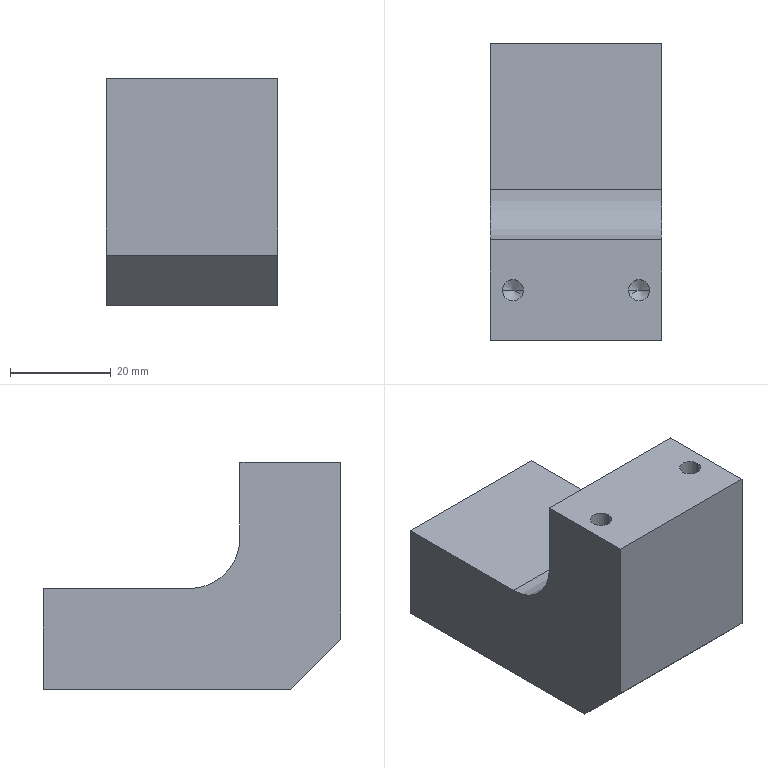Part | SolidWorks | features 3DProfileFeature 2, HoleWzd 2, Chamfer 1, Extrusion 1, Fillet 1, ICE 1 | 1 solid | 26 faces | box 34 x 59 x 45 mm | volume 55439 mm3 | cylinder 9 | plane 9 | cone 8 | commonest cylinder face diameters 4.2 x8 20 x1
STEP:
#1=CARTESIAN_POINT('',(-14.6,10.,10.1));
#2=VERTEX_POINT('',#1);
#3=CARTESIAN_POINT('',(-10.4,10.,10.1));
#4=VERTEX_POINT('',#3);
#5=CARTESIAN_POINT('',(-12.5,10.,10.1));
#6=DIRECTION('',(0.,0.,1.));
#7=DIRECTION('',(1.,0.,0.));
#8=AXIS2_PLACEMENT_3D('',#5,#6,#7);
#9=CIRCLE('',#8,2.1);
#10=EDGE_CURVE('',#2,#4,#9,.T.);
#11=ORIENTED_EDGE('',*,*,#10,.F.);
#12=CARTESIAN_POINT('',(-14.6,10.,22.5));
#13=VERTEX_POINT('',#12);
#14=CARTESIAN_POINT('',(-14.6,10.,22.5));
#15=DIRECTION('',(0.,0.,1.));
#16=VECTOR('',#15,1000.);
#17=LINE('',#14,#16);
#18=EDGE_CURVE('',#2,#13,#17,.T.);
#19=ORIENTED_EDGE('',*,*,#18,.T.);
#20=CARTESIAN_POINT('',(-10.4,10.,22.5));
#21=VERTEX_POINT('',#20);
#22=CARTESIAN_POINT('',(-12.5,10.,22.5));
#23=DIRECTION('',(0.,0.,1.));
#24=DIRECTION('',(1.,0.,0.));
#25=AXIS2_PLACEMENT_3D('',#22,#23,#24);
#26=CIRCLE('',#25,2.1);
#27=EDGE_CURVE('',#13,#21,#26,.T.);
#28=ORIENTED_EDGE('',*,*,#27,.T.);
#29=CARTESIAN_POINT('',(-10.4,10.,22.5));
#30=DIRECTION('',(0.,0.,1.));
#31=VECTOR('',#30,1000.);
#32=LINE('',#29,#31);
#33=EDGE_CURVE('',#4,#21,#32,.T.);
#34=ORIENTED_EDGE('',*,*,#33,.F.);
#35=EDGE_LOOP('',(#11,#19,#28,#34));
#36=FACE_OUTER_BOUND('',#35,.T.);
#37=CARTESIAN_POINT('',(-12.5,10.,22.5));
#38=DIRECTION('',(0.,0.,1.));
#39=DIRECTION('',(1.,0.,0.));
#40=AXIS2_PLACEMENT_3D('',#37,#38,#39);
#41=CYLINDRICAL_SURFACE('',#40,2.1);
#42=ADVANCED_FACE('',(#36),#41,.F.);
#43=CARTESIAN_POINT('',(-12.5,10.,8.838));
#44=VERTEX_POINT('',#43);
#45=CARTESIAN_POINT('',(-10.4,10.,10.1));
#46=DIRECTION('',(0.8572,0.,0.515));
#47=VECTOR('',#46,1000.);
#48=LINE('',#45,#47);
#49=EDGE_CURVE('',#44,#4,#48,.T.);
#50=ORIENTED_EDGE('',*,*,#49,.F.);
#51=CARTESIAN_POINT('',(-14.6,10.,10.1));
#52=DIRECTION('',(-0.8572,0.,0.515));
#53=VECTOR('',#52,1000.);
#54=LINE('',#51,#53);
#55=EDGE_CURVE('',#44,#2,#54,.T.);
#56=ORIENTED_EDGE('',*,*,#55,.T.);
#57=ORIENTED_EDGE('',*,*,#10,.T.);
#58=EDGE_LOOP('',(#50,#56,#57));
#59=FACE_OUTER_BOUND('',#58,.T.);
#60=CARTESIAN_POINT('',(-12.5,10.,10.1));
#61=DIRECTION('',(0.,0.,1.));
#62=DIRECTION('',(1.,0.,0.));
#63=AXIS2_PLACEMENT_3D('',#60,#61,#62);
#64=CONICAL_SURFACE('',#63,2.1,1.03);
#65=ADVANCED_FACE('',(#59),#64,.F.);
#66=CARTESIAN_POINT('',(10.4,10.,10.1));
#67=VERTEX_POINT('',#66);
#68=CARTESIAN_POINT('',(14.6,10.,10.1));
#69=VERTEX_POINT('',#68);
#70=CARTESIAN_POINT('',(12.5,10.,10.1));
#71=DIRECTION('',(0.,0.,1.));
#72=DIRECTION('',(1.,0.,0.));
#73=AXIS2_PLACEMENT_3D('',#70,#71,#72);
#74=CIRCLE('',#73,2.1);
#75=EDGE_CURVE('',#67,#69,#74,.T.);
#76=ORIENTED_EDGE('',*,*,#75,.F.);
#77=CARTESIAN_POINT('',(10.4,10.,22.5));
#78=VERTEX_POINT('',#77);
#79=CARTESIAN_POINT('',(10.4,10.,22.5));
#80=DIRECTION('',(0.,0.,1.));
#81=VECTOR('',#80,1000.);
#82=LINE('',#79,#81);
#83=EDGE_CURVE('',#67,#78,#82,.T.);
#84=ORIENTED_EDGE('',*,*,#83,.T.);
#85=CARTESIAN_POINT('',(14.6,10.,22.5));
#86=VERTEX_POINT('',#85);
#87=CARTESIAN_POINT('',(12.5,10.,22.5));
#88=DIRECTION('',(0.,0.,1.));
#89=DIRECTION('',(1.,0.,0.));
#90=AXIS2_PLACEMENT_3D('',#87,#88,#89);
#91=CIRCLE('',#90,2.1);
#92=EDGE_CURVE('',#78,#86,#91,.T.);
#93=ORIENTED_EDGE('',*,*,#92,.T.);
#94=CARTESIAN_POINT('',(14.6,10.,22.5));
#95=DIRECTION('',(0.,0.,1.));
#96=VECTOR('',#95,1000.);
#97=LINE('',#94,#96);
#98=EDGE_CURVE('',#69,#86,#97,.T.);
#99=ORIENTED_EDGE('',*,*,#98,.F.);
#100=EDGE_LOOP('',(#76,#84,#93,#99));
#101=FACE_OUTER_BOUND('',#100,.T.);
#102=CARTESIAN_POINT('',(12.5,10.,22.5));
#103=DIRECTION('',(0.,0.,1.));
#104=DIRECTION('',(1.,0.,0.));
#105=AXIS2_PLACEMENT_3D('',#102,#103,#104);
#106=CYLINDRICAL_SURFACE('',#105,2.1);
#107=ADVANCED_FACE('',(#101),#106,.F.);
#108=CARTESIAN_POINT('',(12.5,10.,8.838));
#109=VERTEX_POINT('',#108);
#110=CARTESIAN_POINT('',(14.6,10.,10.1));
#111=DIRECTION('',(0.8572,0.,0.515));
#112=VECTOR('',#111,1000.);
#113=LINE('',#110,#112);
#114=EDGE_CURVE('',#109,#69,#113,.T.);
#115=ORIENTED_EDGE('',*,*,#114,.F.);
#116=CARTESIAN_POINT('',(10.4,10.,10.1));
#117=DIRECTION('',(-0.8572,0.,0.515));
#118=VECTOR('',#117,1000.);
#119=LINE('',#116,#118);
#120=EDGE_CURVE('',#109,#67,#119,.T.);
#121=ORIENTED_EDGE('',*,*,#120,.T.);
#122=ORIENTED_EDGE('',*,*,#75,.T.);
#123=EDGE_LOOP('',(#115,#121,#122));
#124=FACE_OUTER_BOUND('',#123,.T.);
#125=CARTESIAN_POINT('',(12.5,10.,10.1));
#126=DIRECTION('',(0.,0.,1.));
#127=DIRECTION('',(1.,0.,0.));
#128=AXIS2_PLACEMENT_3D('',#125,#126,#127);
#129=CONICAL_SURFACE('',#128,2.1,1.03);
#130=ADVANCED_FACE('',(#124),#129,.F.);
#131=CARTESIAN_POINT('',(-11.,46.6,-14.6));
#132=VERTEX_POINT('',#131);
#133=CARTESIAN_POINT('',(-11.,46.6,-10.4));
#134=VERTEX_POINT('',#133);
#135=CARTESIAN_POINT('',(-11.,46.6,-12.5));
#136=DIRECTION('',(0.,1.,0.));
#137=DIRECTION('',(0.,0.,1.));
#138=AXIS2_PLACEMENT_3D('',#135,#136,#137);
#139=CIRCLE('',#138,2.1);
#140=EDGE_CURVE('',#132,#134,#139,.T.);
#141=ORIENTED_EDGE('',*,*,#140,.F.);
#142=CARTESIAN_POINT('',(-11.,59.,-14.6));
#143=VERTEX_POINT('',#142);
#144=CARTESIAN_POINT('',(-11.,59.,-14.6));
#145=DIRECTION('',(0.,1.,0.));
#146=VECTOR('',#145,1000.);
#147=LINE('',#144,#146);
#148=EDGE_CURVE('',#132,#143,#147,.T.);
#149=ORIENTED_EDGE('',*,*,#148,.T.);
#150=CARTESIAN_POINT('',(-11.,59.,-10.4));
#151=VERTEX_POINT('',#150);
#152=CARTESIAN_POINT('',(-11.,59.,-12.5));
#153=DIRECTION('',(0.,1.,0.));
#154=DIRECTION('',(0.,0.,1.));
#155=AXIS2_PLACEMENT_3D('',#152,#153,#154);
#156=CIRCLE('',#155,2.1);
#157=EDGE_CURVE('',#143,#151,#156,.T.);
#158=ORIENTED_EDGE('',*,*,#157,.T.);
#159=CARTESIAN_POINT('',(-11.,59.,-10.4));
#160=DIRECTION('',(0.,1.,0.));
#161=VECTOR('',#160,1000.);
#162=LINE('',#159,#161);
#163=EDGE_CURVE('',#134,#151,#162,.T.);
#164=ORIENTED_EDGE('',*,*,#163,.F.);
#165=EDGE_LOOP('',(#141,#149,#158,#164));
#166=FACE_OUTER_BOUND('',#165,.T.);
#167=CARTESIAN_POINT('',(-11.,59.,-12.5));
#168=DIRECTION('',(0.,1.,0.));
#169=DIRECTION('',(0.,0.,1.));
#170=AXIS2_PLACEMENT_3D('',#167,#168,#169);
#171=CYLINDRICAL_SURFACE('',#170,2.1);
#172=ADVANCED_FACE('',(#166),#171,.F.);
#173=CARTESIAN_POINT('',(-11.,45.338,-12.5));
#174=VERTEX_POINT('',#173);
#175=CARTESIAN_POINT('',(-11.,46.6,-10.4));
#176=DIRECTION('',(0.,0.515,0.8572));
#177=VECTOR('',#176,1000.);
#178=LINE('',#175,#177);
#179=EDGE_CURVE('',#174,#134,#178,.T.);
#180=ORIENTED_EDGE('',*,*,#179,.F.);
#181=CARTESIAN_POINT('',(-11.,46.6,-14.6));
#182=DIRECTION('',(0.,0.515,-0.8572));
#183=VECTOR('',#182,1000.);
#184=LINE('',#181,#183);
#185=EDGE_CURVE('',#174,#132,#184,.T.);
#186=ORIENTED_EDGE('',*,*,#185,.T.);
#187=ORIENTED_EDGE('',*,*,#140,.T.);
#188=EDGE_LOOP('',(#180,#186,#187));
#189=FACE_OUTER_BOUND('',#188,.T.);
#190=CARTESIAN_POINT('',(-11.,46.6,-12.5));
#191=DIRECTION('',(0.,1.,0.));
#192=DIRECTION('',(0.,0.,1.));
#193=AXIS2_PLACEMENT_3D('',#190,#191,#192);
#194=CONICAL_SURFACE('',#193,2.1,1.03);
#195=ADVANCED_FACE('',(#189),#194,.F.);
#196=CARTESIAN_POINT('',(11.,46.6,-14.6));
#197=VERTEX_POINT('',#196);
#198=CARTESIAN_POINT('',(11.,46.6,-10.4));
#199=VERTEX_POINT('',#198);
#200=CARTESIAN_POINT('',(11.,46.6,-12.5));
#201=DIRECTION('',(0.,1.,0.));
#202=DIRECTION('',(0.,0.,1.));
#203=AXIS2_PLACEMENT_3D('',#200,#201,#202);
#204=CIRCLE('',#203,2.1);
#205=EDGE_CURVE('',#197,#199,#204,.T.);
#206=ORIENTED_EDGE('',*,*,#205,.F.);
#207=CARTESIAN_POINT('',(11.,59.,-14.6));
#208=VERTEX_POINT('',#207);
#209=CARTESIAN_POINT('',(11.,59.,-14.6));
#210=DIRECTION('',(0.,1.,0.));
#211=VECTOR('',#210,1000.);
#212=LINE('',#209,#211);
#213=EDGE_CURVE('',#197,#208,#212,.T.);
#214=ORIENTED_EDGE('',*,*,#213,.T.);
#215=CARTESIAN_POINT('',(11.,59.,-10.4));
#216=VERTEX_POINT('',#215);
#217=CARTESIAN_POINT('',(11.,59.,-12.5));
#218=DIRECTION('',(0.,1.,0.));
#219=DIRECTION('',(0.,0.,1.));
#220=AXIS2_PLACEMENT_3D('',#217,#218,#219);
#221=CIRCLE('',#220,2.1);
#222=EDGE_CURVE('',#208,#216,#221,.T.);
#223=ORIENTED_EDGE('',*,*,#222,.T.);
#224=CARTESIAN_POINT('',(11.,59.,-10.4));
#225=DIRECTION('',(0.,1.,0.));
#226=VECTOR('',#225,1000.);
#227=LINE('',#224,#226);
#228=EDGE_CURVE('',#199,#216,#227,.T.);
#229=ORIENTED_EDGE('',*,*,#228,.F.);
#230=EDGE_LOOP('',(#206,#214,#223,#229));
#231=FACE_OUTER_BOUND('',#230,.T.);
#232=CARTESIAN_POINT('',(11.,59.,-12.5));
#233=DIRECTION('',(0.,1.,0.));
#234=DIRECTION('',(0.,0.,1.));
#235=AXIS2_PLACEMENT_3D('',#232,#233,#234);
#236=CYLINDRICAL_SURFACE('',#235,2.1);
#237=ADVANCED_FACE('',(#231),#236,.F.);
#238=CARTESIAN_POINT('',(11.,45.338,-12.5));
#239=VERTEX_POINT('',#238);
#240=CARTESIAN_POINT('',(11.,46.6,-10.4));
#241=DIRECTION('',(0.,0.515,0.8572));
#242=VECTOR('',#241,1000.);
#243=LINE('',#240,#242);
#244=EDGE_CURVE('',#239,#199,#243,.T.);
#245=ORIENTED_EDGE('',*,*,#244,.F.);
#246=CARTESIAN_POINT('',(11.,46.6,-14.6));
#247=DIRECTION('',(0.,0.515,-0.8572));
#248=VECTOR('',#247,1000.);
#249=LINE('',#246,#248);
#250=EDGE_CURVE('',#239,#197,#249,.T.);
#251=ORIENTED_EDGE('',*,*,#250,.T.);
#252=ORIENTED_EDGE('',*,*,#205,.T.);
#253=EDGE_LOOP('',(#245,#251,#252));
#254=FACE_OUTER_BOUND('',#253,.T.);
#255=CARTESIAN_POINT('',(11.,46.6,-12.5));
#256=DIRECTION('',(0.,1.,0.));
#257=DIRECTION('',(0.,0.,1.));
#258=AXIS2_PLACEMENT_3D('',#255,#256,#257);
#259=CONICAL_SURFACE('',#258,2.1,1.03);
#260=ADVANCED_FACE('',(#254),#259,.F.);
#261=CARTESIAN_POINT('',(17.,0.,22.5));
#262=VERTEX_POINT('',#261);
#263=CARTESIAN_POINT('',(17.,0.,-12.5));
#264=VERTEX_POINT('',#263);
#265=CARTESIAN_POINT('',(17.,0.,-22.5));
#266=DIRECTION('',(0.,0.,-1.));
#267=VECTOR('',#266,1000.);
#268=LINE('',#265,#267);
#269=EDGE_CURVE('',#262,#264,#268,.T.);
#270=ORIENTED_EDGE('',*,*,#269,.T.);
#271=CARTESIAN_POINT('',(17.,10.,-22.5));
#272=VERTEX_POINT('',#271);
#273=CARTESIAN_POINT('',(17.,10.,-22.5));
#274=DIRECTION('',(0.,0.7071,-0.7071));
#275=VECTOR('',#274,1000.);
#276=LINE('',#273,#275);
#277=EDGE_CURVE('',#264,#272,#276,.T.);
#278=ORIENTED_EDGE('',*,*,#277,.T.);
#279=CARTESIAN_POINT('',(17.,59.,-22.5));
#280=VERTEX_POINT('',#279);
#281=CARTESIAN_POINT('',(17.,59.,-22.5));
#282=DIRECTION('',(0.,-1.,0.));
#283=VECTOR('',#282,1000.);
#284=LINE('',#281,#283);
#285=EDGE_CURVE('',#280,#272,#284,.T.);
#286=ORIENTED_EDGE('',*,*,#285,.F.);
#287=CARTESIAN_POINT('',(17.,59.,-2.5));
#288=VERTEX_POINT('',#287);
#289=CARTESIAN_POINT('',(17.,59.,-22.5));
#290=DIRECTION('',(0.,0.,-1.));
#291=VECTOR('',#290,1000.);
#292=LINE('',#289,#291);
#293=EDGE_CURVE('',#288,#280,#292,.T.);
#294=ORIENTED_EDGE('',*,*,#293,.F.);
#295=CARTESIAN_POINT('',(17.,30.,-2.5));
#296=VERTEX_POINT('',#295);
#297=CARTESIAN_POINT('',(17.,59.,-2.5));
#298=DIRECTION('',(0.,1.,0.));
#299=VECTOR('',#298,1000.);
#300=LINE('',#297,#299);
#301=EDGE_CURVE('',#296,#288,#300,.T.);
#302=ORIENTED_EDGE('',*,*,#301,.F.);
#303=CARTESIAN_POINT('',(17.,20.,7.5));
#304=VERTEX_POINT('',#303);
#305=CARTESIAN_POINT('',(17.,30.,7.5));
#306=DIRECTION('',(-1.,0.,0.));
#307=DIRECTION('',(0.,0.,1.));
#308=AXIS2_PLACEMENT_3D('',#305,#306,#307);
#309=CIRCLE('',#308,10.);
#310=EDGE_CURVE('',#296,#304,#309,.T.);
#311=ORIENTED_EDGE('',*,*,#310,.T.);
#312=CARTESIAN_POINT('',(17.,20.,22.5));
#313=VERTEX_POINT('',#312);
#314=CARTESIAN_POINT('',(17.,20.,22.5));
#315=DIRECTION('',(0.,0.,-1.));
#316=VECTOR('',#315,1000.);
#317=LINE('',#314,#316);
#318=EDGE_CURVE('',#313,#304,#317,.T.);
#319=ORIENTED_EDGE('',*,*,#318,.F.);
#320=CARTESIAN_POINT('',(17.,59.,22.5));
#321=DIRECTION('',(0.,-1.,0.));
#322=VECTOR('',#321,1000.);
#323=LINE('',#320,#322);
#324=EDGE_CURVE('',#313,#262,#323,.T.);
#325=ORIENTED_EDGE('',*,*,#324,.T.);
#326=EDGE_LOOP('',(#270,#278,#286,#294,#302,#311,#319,#325));
#327=FACE_OUTER_BOUND('',#326,.T.);
#328=CARTESIAN_POINT('',(17.,59.,-22.5));
#329=DIRECTION('',(-1.,0.,0.));
#330=DIRECTION('',(0.,0.,1.));
#331=AXIS2_PLACEMENT_3D('',#328,#329,#330);
#332=PLANE('',#331);
#333=ADVANCED_FACE('',(#327),#332,.F.);
#334=ORIENTED_EDGE('',*,*,#285,.T.);
#335=CARTESIAN_POINT('',(-17.,10.,-22.5));
#336=VERTEX_POINT('',#335);
#337=CARTESIAN_POINT('',(-17.,10.,-22.5));
#338=DIRECTION('',(-1.,0.,0.));
#339=VECTOR('',#338,1000.);
#340=LINE('',#337,#339);
#341=EDGE_CURVE('',#272,#336,#340,.T.);
#342=ORIENTED_EDGE('',*,*,#341,.T.);
#343=CARTESIAN_POINT('',(-17.,59.,-22.5));
#344=VERTEX_POINT('',#343);
#345=CARTESIAN_POINT('',(-17.,59.,-22.5));
#346=DIRECTION('',(0.,-1.,0.));
#347=VECTOR('',#346,1000.);
#348=LINE('',#345,#347);
#349=EDGE_CURVE('',#344,#336,#348,.T.);
#350=ORIENTED_EDGE('',*,*,#349,.F.);
#351=CARTESIAN_POINT('',(-17.,59.,-22.5));
#352=DIRECTION('',(-1.,0.,0.));
#353=VECTOR('',#352,1000.);
#354=LINE('',#351,#353);
#355=EDGE_CURVE('',#280,#344,#354,.T.);
#356=ORIENTED_EDGE('',*,*,#355,.F.);
#357=EDGE_LOOP('',(#334,#342,#350,#356));
#358=FACE_OUTER_BOUND('',#357,.T.);
#359=CARTESIAN_POINT('',(-17.,59.,-22.5));
#360=DIRECTION('',(0.,0.,1.));
#361=DIRECTION('',(1.,0.,0.));
#362=AXIS2_PLACEMENT_3D('',#359,#360,#361);
#363=PLANE('',#362);
#364=ADVANCED_FACE('',(#358),#363,.F.);
#365=ORIENTED_EDGE('',*,*,#349,.T.);
#366=CARTESIAN_POINT('',(-17.,0.,-12.5));
#367=VERTEX_POINT('',#366);
#368=CARTESIAN_POINT('',(-17.,10.,-22.5));
#369=DIRECTION('',(0.,-0.7071,0.7071));
#370=VECTOR('',#369,1000.);
#371=LINE('',#368,#370);
#372=EDGE_CURVE('',#336,#367,#371,.T.);
#373=ORIENTED_EDGE('',*,*,#372,.T.);
#374=CARTESIAN_POINT('',(-17.,0.,22.5));
#375=VERTEX_POINT('',#374);
#376=CARTESIAN_POINT('',(-17.,0.,-22.5));
#377=DIRECTION('',(0.,0.,1.));
#378=VECTOR('',#377,1000.);
#379=LINE('',#376,#378);
#380=EDGE_CURVE('',#367,#375,#379,.T.);
#381=ORIENTED_EDGE('',*,*,#380,.T.);
#382=CARTESIAN_POINT('',(-17.,20.,22.5));
#383=VERTEX_POINT('',#382);
#384=CARTESIAN_POINT('',(-17.,59.,22.5));
#385=DIRECTION('',(0.,-1.,0.));
#386=VECTOR('',#385,1000.);
#387=LINE('',#384,#386);
#388=EDGE_CURVE('',#383,#375,#387,.T.);
#389=ORIENTED_EDGE('',*,*,#388,.F.);
#390=CARTESIAN_POINT('',(-17.,20.,7.5));
#391=VERTEX_POINT('',#390);
#392=CARTESIAN_POINT('',(-17.,20.,-22.5));
#393=DIRECTION('',(0.,0.,-1.));
#394=VECTOR('',#393,1000.);
#395=LINE('',#392,#394);
#396=EDGE_CURVE('',#383,#391,#395,.T.);
#397=ORIENTED_EDGE('',*,*,#396,.T.);
#398=CARTESIAN_POINT('',(-17.,30.,-2.5));
#399=VERTEX_POINT('',#398);
#400=CARTESIAN_POINT('',(-17.,30.,7.5));
#401=DIRECTION('',(1.,0.,0.));
#402=DIRECTION('',(0.,0.,-1.));
#403=AXIS2_PLACEMENT_3D('',#400,#401,#402);
#404=CIRCLE('',#403,10.);
#405=EDGE_CURVE('',#391,#399,#404,.T.);
#406=ORIENTED_EDGE('',*,*,#405,.T.);
#407=CARTESIAN_POINT('',(-17.,59.,-2.5));
#408=VERTEX_POINT('',#407);
#409=CARTESIAN_POINT('',(-17.,59.,-2.5));
#410=DIRECTION('',(0.,1.,0.));
#411=VECTOR('',#410,1000.);
#412=LINE('',#409,#411);
#413=EDGE_CURVE('',#399,#408,#412,.T.);
#414=ORIENTED_EDGE('',*,*,#413,.T.);
#415=CARTESIAN_POINT('',(-17.,59.,-22.5));
#416=DIRECTION('',(0.,0.,1.));
#417=VECTOR('',#416,1000.);
#418=LINE('',#415,#417);
#419=EDGE_CURVE('',#344,#408,#418,.T.);
#420=ORIENTED_EDGE('',*,*,#419,.F.);
#421=EDGE_LOOP('',(#365,#373,#381,#389,#397,#406,#414,#420));
#422=FACE_OUTER_BOUND('',#421,.T.);
#423=CARTESIAN_POINT('',(-17.,59.,-22.5));
#424=DIRECTION('',(1.,0.,0.));
#425=DIRECTION('',(0.,0.,-1.));
#426=AXIS2_PLACEMENT_3D('',#423,#424,#425);
#427=PLANE('',#426);
#428=ADVANCED_FACE('',(#422),#427,.F.);
#429=CARTESIAN_POINT('',(-12.5,10.,22.5));
#430=DIRECTION('',(0.,0.,1.));
#431=DIRECTION('',(1.,0.,0.));
#432=AXIS2_PLACEMENT_3D('',#429,#430,#431);
#433=CIRCLE('',#432,2.1);
#434=EDGE_CURVE('',#21,#13,#433,.T.);
#435=ORIENTED_EDGE('',*,*,#434,.F.);
#436=ORIENTED_EDGE('',*,*,#27,.F.);
#437=EDGE_LOOP('',(#435,#436));
#438=FACE_BOUND('',#437,.T.);
#439=CARTESIAN_POINT('',(12.5,10.,22.5));
#440=DIRECTION('',(0.,0.,1.));
#441=DIRECTION('',(1.,0.,0.));
#442=AXIS2_PLACEMENT_3D('',#439,#440,#441);
#443=CIRCLE('',#442,2.1);
#444=EDGE_CURVE('',#86,#78,#443,.T.);
#445=ORIENTED_EDGE('',*,*,#444,.F.);
#446=ORIENTED_EDGE('',*,*,#92,.F.);
#447=EDGE_LOOP('',(#445,#446));
#448=FACE_BOUND('',#447,.T.);
#449=ORIENTED_EDGE('',*,*,#324,.F.);
#450=CARTESIAN_POINT('',(-28.,20.,22.5));
#451=DIRECTION('',(1.,0.,0.));
#452=VECTOR('',#451,1000.);
#453=LINE('',#450,#452);
#454=EDGE_CURVE('',#383,#313,#453,.T.);
#455=ORIENTED_EDGE('',*,*,#454,.F.);
#456=ORIENTED_EDGE('',*,*,#388,.T.);
#457=CARTESIAN_POINT('',(-17.,0.,22.5));
#458=DIRECTION('',(1.,0.,0.));
#459=VECTOR('',#458,1000.);
#460=LINE('',#457,#459);
#461=EDGE_CURVE('',#375,#262,#460,.T.);
#462=ORIENTED_EDGE('',*,*,#461,.T.);
#463=EDGE_LOOP('',(#449,#455,#456,#462));
#464=FACE_OUTER_BOUND('',#463,.T.);
#465=CARTESIAN_POINT('',(-17.,59.,22.5));
#466=DIRECTION('',(0.,0.,-1.));
#467=DIRECTION('',(-1.,0.,0.));
#468=AXIS2_PLACEMENT_3D('',#465,#466,#467);
#469=PLANE('',#468);
#470=ADVANCED_FACE('',(#438,#448,#464),#469,.F.);
#471=CARTESIAN_POINT('',(-11.,59.,-12.5));
#472=DIRECTION('',(0.,1.,0.));
#473=DIRECTION('',(0.,0.,1.));
#474=AXIS2_PLACEMENT_3D('',#471,#472,#473);
#475=CIRCLE('',#474,2.1);
#476=EDGE_CURVE('',#151,#143,#475,.T.);
#477=ORIENTED_EDGE('',*,*,#476,.F.);
#478=ORIENTED_EDGE('',*,*,#157,.F.);
#479=EDGE_LOOP('',(#477,#478));
#480=FACE_BOUND('',#479,.T.);
#481=CARTESIAN_POINT('',(11.,59.,-12.5));
#482=DIRECTION('',(0.,1.,0.));
#483=DIRECTION('',(0.,0.,1.));
#484=AXIS2_PLACEMENT_3D('',#481,#482,#483);
#485=CIRCLE('',#484,2.1);
#486=EDGE_CURVE('',#216,#208,#485,.T.);
#487=ORIENTED_EDGE('',*,*,#486,.F.);
#488=ORIENTED_EDGE('',*,*,#222,.F.);
#489=EDGE_LOOP('',(#487,#488));
#490=FACE_BOUND('',#489,.T.);
#491=CARTESIAN_POINT('',(0.,59.,-2.5));
#492=DIRECTION('',(-1.,0.,0.));
#493=VECTOR('',#492,1000.);
#494=LINE('',#491,#493);
#495=EDGE_CURVE('',#288,#408,#494,.T.);
#496=ORIENTED_EDGE('',*,*,#495,.F.);
#497=ORIENTED_EDGE('',*,*,#293,.T.);
#498=ORIENTED_EDGE('',*,*,#355,.T.);
#499=ORIENTED_EDGE('',*,*,#419,.T.);
#500=EDGE_LOOP('',(#496,#497,#498,#499));
#501=FACE_OUTER_BOUND('',#500,.T.);
#502=CARTESIAN_POINT('',(0.,59.,0.));
#503=DIRECTION('',(0.,1.,0.));
#504=DIRECTION('',(0.,0.,1.));
#505=AXIS2_PLACEMENT_3D('',#502,#503,#504);
#506=PLANE('',#505);
#507=ADVANCED_FACE('',(#480,#490,#501),#506,.T.);
#508=ORIENTED_EDGE('',*,*,#380,.F.);
#509=CARTESIAN_POINT('',(0.,0.,-12.5));
#510=DIRECTION('',(1.,0.,0.));
#511=VECTOR('',#510,1000.);
#512=LINE('',#509,#511);
#513=EDGE_CURVE('',#367,#264,#512,.T.);
#514=ORIENTED_EDGE('',*,*,#513,.T.);
#515=ORIENTED_EDGE('',*,*,#269,.F.);
#516=ORIENTED_EDGE('',*,*,#461,.F.);
#517=EDGE_LOOP('',(#508,#514,#515,#516));
#518=FACE_OUTER_BOUND('',#517,.T.);
#519=CARTESIAN_POINT('',(0.,0.,0.));
#520=DIRECTION('',(0.,1.,0.));
#521=DIRECTION('',(0.,0.,1.));
#522=AXIS2_PLACEMENT_3D('',#519,#520,#521);
#523=PLANE('',#522);
#524=ADVANCED_FACE('',(#518),#523,.F.);
#525=ORIENTED_EDGE('',*,*,#318,.T.);
#526=CARTESIAN_POINT('',(-17.,20.,7.5));
#527=DIRECTION('',(-1.,0.,0.));
#528=VECTOR('',#527,1000.);
#529=LINE('',#526,#528);
#530=EDGE_CURVE('',#304,#391,#529,.T.);
#531=ORIENTED_EDGE('',*,*,#530,.T.);
#532=ORIENTED_EDGE('',*,*,#396,.F.);
#533=ORIENTED_EDGE('',*,*,#454,.T.);
#534=EDGE_LOOP('',(#525,#531,#532,#533));
#535=FACE_OUTER_BOUND('',#534,.T.);
#536=CARTESIAN_POINT('',(-28.,20.,22.5));
#537=DIRECTION('',(0.,-1.,0.));
#538=DIRECTION('',(0.,0.,-1.));
#539=AXIS2_PLACEMENT_3D('',#536,#537,#538);
#540=PLANE('',#539);
#541=ADVANCED_FACE('',(#535),#540,.F.);
#542=ORIENTED_EDGE('',*,*,#413,.F.);
#543=CARTESIAN_POINT('',(17.,30.,-2.5));
#544=DIRECTION('',(1.,0.,0.));
#545=VECTOR('',#544,1000.);
#546=LINE('',#543,#545);
#547=EDGE_CURVE('',#399,#296,#546,.T.);
#548=ORIENTED_EDGE('',*,*,#547,.T.);
#549=ORIENTED_EDGE('',*,*,#301,.T.);
#550=ORIENTED_EDGE('',*,*,#495,.T.);
#551=EDGE_LOOP('',(#542,#548,#549,#550));
#552=FACE_OUTER_BOUND('',#551,.T.);
#553=CARTESIAN_POINT('',(-28.,59.,-2.5));
#554=DIRECTION('',(0.,0.,-1.));
#555=DIRECTION('',(-1.,0.,0.));
#556=AXIS2_PLACEMENT_3D('',#553,#554,#555);
#557=PLANE('',#556);
#558=ADVANCED_FACE('',(#552),#557,.F.);
#559=ORIENTED_EDGE('',*,*,#277,.F.);
#560=ORIENTED_EDGE('',*,*,#513,.F.);
#561=ORIENTED_EDGE('',*,*,#372,.F.);
#562=ORIENTED_EDGE('',*,*,#341,.F.);
#563=EDGE_LOOP('',(#559,#560,#561,#562));
#564=FACE_OUTER_BOUND('',#563,.T.);
#565=CARTESIAN_POINT('',(-17.,10.,-22.5));
#566=DIRECTION('',(0.,0.7071,0.7071));
#567=DIRECTION('',(-1.,0.,0.));
#568=AXIS2_PLACEMENT_3D('',#565,#566,#567);
#569=PLANE('',#568);
#570=ADVANCED_FACE('',(#564),#569,.F.);
#571=ORIENTED_EDGE('',*,*,#405,.F.);
#572=ORIENTED_EDGE('',*,*,#530,.F.);
#573=ORIENTED_EDGE('',*,*,#310,.F.);
#574=ORIENTED_EDGE('',*,*,#547,.F.);
#575=EDGE_LOOP('',(#571,#572,#573,#574));
#576=FACE_OUTER_BOUND('',#575,.T.);
#577=CARTESIAN_POINT('',(-28.,30.,7.5));
#578=DIRECTION('',(-1.,0.,0.));
#579=DIRECTION('',(0.,0.,1.));
#580=AXIS2_PLACEMENT_3D('',#577,#578,#579);
#581=CYLINDRICAL_SURFACE('',#580,10.);
#582=ADVANCED_FACE('',(#576),#581,.F.);
#583=ORIENTED_EDGE('',*,*,#250,.F.);
#584=ORIENTED_EDGE('',*,*,#244,.T.);
#585=CARTESIAN_POINT('',(11.,46.6,-12.5));
#586=DIRECTION('',(0.,1.,0.));
#587=DIRECTION('',(0.,0.,1.));
#588=AXIS2_PLACEMENT_3D('',#585,#586,#587);
#589=CIRCLE('',#588,2.1);
#590=EDGE_CURVE('',#199,#197,#589,.T.);
#591=ORIENTED_EDGE('',*,*,#590,.T.);
#592=EDGE_LOOP('',(#583,#584,#591));
#593=FACE_OUTER_BOUND('',#592,.T.);
#594=CARTESIAN_POINT('',(11.,46.6,-12.5));
#595=DIRECTION('',(0.,1.,0.));
#596=DIRECTION('',(0.,0.,1.));
#597=AXIS2_PLACEMENT_3D('',#594,#595,#596);
#598=CONICAL_SURFACE('',#597,2.1,1.03);
#599=ADVANCED_FACE('',(#593),#598,.F.);
#600=ORIENTED_EDGE('',*,*,#213,.F.);
#601=ORIENTED_EDGE('',*,*,#590,.F.);
#602=ORIENTED_EDGE('',*,*,#228,.T.);
#603=ORIENTED_EDGE('',*,*,#486,.T.);
#604=EDGE_LOOP('',(#600,#601,#602,#603));
#605=FACE_OUTER_BOUND('',#604,.T.);
#606=CARTESIAN_POINT('',(11.,59.,-12.5));
#607=DIRECTION('',(0.,1.,0.));
#608=DIRECTION('',(0.,0.,1.));
#609=AXIS2_PLACEMENT_3D('',#606,#607,#608);
#610=CYLINDRICAL_SURFACE('',#609,2.1);
#611=ADVANCED_FACE('',(#605),#610,.F.);
#612=ORIENTED_EDGE('',*,*,#185,.F.);
#613=ORIENTED_EDGE('',*,*,#179,.T.);
#614=CARTESIAN_POINT('',(-11.,46.6,-12.5));
#615=DIRECTION('',(0.,1.,0.));
#616=DIRECTION('',(0.,0.,1.));
#617=AXIS2_PLACEMENT_3D('',#614,#615,#616);
#618=CIRCLE('',#617,2.1);
#619=EDGE_CURVE('',#134,#132,#618,.T.);
#620=ORIENTED_EDGE('',*,*,#619,.T.);
#621=EDGE_LOOP('',(#612,#613,#620));
#622=FACE_OUTER_BOUND('',#621,.T.);
#623=CARTESIAN_POINT('',(-11.,46.6,-12.5));
#624=DIRECTION('',(0.,1.,0.));
#625=DIRECTION('',(0.,0.,1.));
#626=AXIS2_PLACEMENT_3D('',#623,#624,#625);
#627=CONICAL_SURFACE('',#626,2.1,1.03);
#628=ADVANCED_FACE('',(#622),#627,.F.);
#629=ORIENTED_EDGE('',*,*,#148,.F.);
#630=ORIENTED_EDGE('',*,*,#619,.F.);
#631=ORIENTED_EDGE('',*,*,#163,.T.);
#632=ORIENTED_EDGE('',*,*,#476,.T.);
#633=EDGE_LOOP('',(#629,#630,#631,#632));
#634=FACE_OUTER_BOUND('',#633,.T.);
#635=CARTESIAN_POINT('',(-11.,59.,-12.5));
#636=DIRECTION('',(0.,1.,0.));
#637=DIRECTION('',(0.,0.,1.));
#638=AXIS2_PLACEMENT_3D('',#635,#636,#637);
#639=CYLINDRICAL_SURFACE('',#638,2.1);
#640=ADVANCED_FACE('',(#634),#639,.F.);
#641=ORIENTED_EDGE('',*,*,#120,.F.);
#642=ORIENTED_EDGE('',*,*,#114,.T.);
#643=CARTESIAN_POINT('',(12.5,10.,10.1));
#644=DIRECTION('',(0.,0.,1.));
#645=DIRECTION('',(1.,0.,0.));
#646=AXIS2_PLACEMENT_3D('',#643,#644,#645);
#647=CIRCLE('',#646,2.1);
#648=EDGE_CURVE('',#69,#67,#647,.T.);
#649=ORIENTED_EDGE('',*,*,#648,.T.);
#650=EDGE_LOOP('',(#641,#642,#649));
#651=FACE_OUTER_BOUND('',#650,.T.);
#652=CARTESIAN_POINT('',(12.5,10.,10.1));
#653=DIRECTION('',(0.,0.,1.));
#654=DIRECTION('',(1.,0.,0.));
#655=AXIS2_PLACEMENT_3D('',#652,#653,#654);
#656=CONICAL_SURFACE('',#655,2.1,1.03);
#657=ADVANCED_FACE('',(#651),#656,.F.);
#658=ORIENTED_EDGE('',*,*,#83,.F.);
#659=ORIENTED_EDGE('',*,*,#648,.F.);
#660=ORIENTED_EDGE('',*,*,#98,.T.);
#661=ORIENTED_EDGE('',*,*,#444,.T.);
#662=EDGE_LOOP('',(#658,#659,#660,#661));
#663=FACE_OUTER_BOUND('',#662,.T.);
#664=CARTESIAN_POINT('',(12.5,10.,22.5));
#665=DIRECTION('',(0.,0.,1.));
#666=DIRECTION('',(1.,0.,0.));
#667=AXIS2_PLACEMENT_3D('',#664,#665,#666);
#668=CYLINDRICAL_SURFACE('',#667,2.1);
#669=ADVANCED_FACE('',(#663),#668,.F.);
#670=ORIENTED_EDGE('',*,*,#55,.F.);
#671=ORIENTED_EDGE('',*,*,#49,.T.);
#672=CARTESIAN_POINT('',(-12.5,10.,10.1));
#673=DIRECTION('',(0.,0.,1.));
#674=DIRECTION('',(1.,0.,0.));
#675=AXIS2_PLACEMENT_3D('',#672,#673,#674);
#676=CIRCLE('',#675,2.1);
#677=EDGE_CURVE('',#4,#2,#676,.T.);
#678=ORIENTED_EDGE('',*,*,#677,.T.);
#679=EDGE_LOOP('',(#670,#671,#678));
#680=FACE_OUTER_BOUND('',#679,.T.);
#681=CARTESIAN_POINT('',(-12.5,10.,10.1));
#682=DIRECTION('',(0.,0.,1.));
#683=DIRECTION('',(1.,0.,0.));
#684=AXIS2_PLACEMENT_3D('',#681,#682,#683);
#685=CONICAL_SURFACE('',#684,2.1,1.03);
#686=ADVANCED_FACE('',(#680),#685,.F.);
#687=ORIENTED_EDGE('',*,*,#18,.F.);
#688=ORIENTED_EDGE('',*,*,#677,.F.);
#689=ORIENTED_EDGE('',*,*,#33,.T.);
#690=ORIENTED_EDGE('',*,*,#434,.T.);
#691=EDGE_LOOP('',(#687,#688,#689,#690));
#692=FACE_OUTER_BOUND('',#691,.T.);
#693=CARTESIAN_POINT('',(-12.5,10.,22.5));
#694=DIRECTION('',(0.,0.,1.));
#695=DIRECTION('',(1.,0.,0.));
#696=AXIS2_PLACEMENT_3D('',#693,#694,#695);
#697=CYLINDRICAL_SURFACE('',#696,2.1);
#698=ADVANCED_FACE('',(#692),#697,.F.);
#699=CLOSED_SHELL('',(#42,#65,#107,#130,#172,#195,#237,#260,#333,#364,#428,#470,#507,#524,#541,#558,#570,#582,#599,#611,#628,#640,#657,#669,#686,#698));
#700=MANIFOLD_SOLID_BREP('',#699);
#701=CARTESIAN_POINT('',(0.,0.,0.));
#702=DIRECTION('',(0.,0.,1.));
#703=DIRECTION('',(1.,0.,0.));
#704=AXIS2_PLACEMENT_3D('',#701,#702,#703);
#705=(LENGTH_UNIT()NAMED_UNIT(*)SI_UNIT(.MILLI.,.METRE.));
#706=UNCERTAINTY_MEASURE_WITH_UNIT(LENGTH_MEASURE(0.00001),#705,'','');
#707=(NAMED_UNIT(*)PLANE_ANGLE_UNIT()SI_UNIT($,.RADIAN.));
#708=(NAMED_UNIT(*)SI_UNIT($,.STERADIAN.)SOLID_ANGLE_UNIT());
#709=(GEOMETRIC_REPRESENTATION_CONTEXT(3)GLOBAL_UNCERTAINTY_ASSIGNED_CONTEXT((#706))GLOBAL_UNIT_ASSIGNED_CONTEXT((#705,#707,#708))REPRESENTATION_CONTEXT('',''));
#710=ADVANCED_BREP_SHAPE_REPRESENTATION('',(#700,#704),#709);